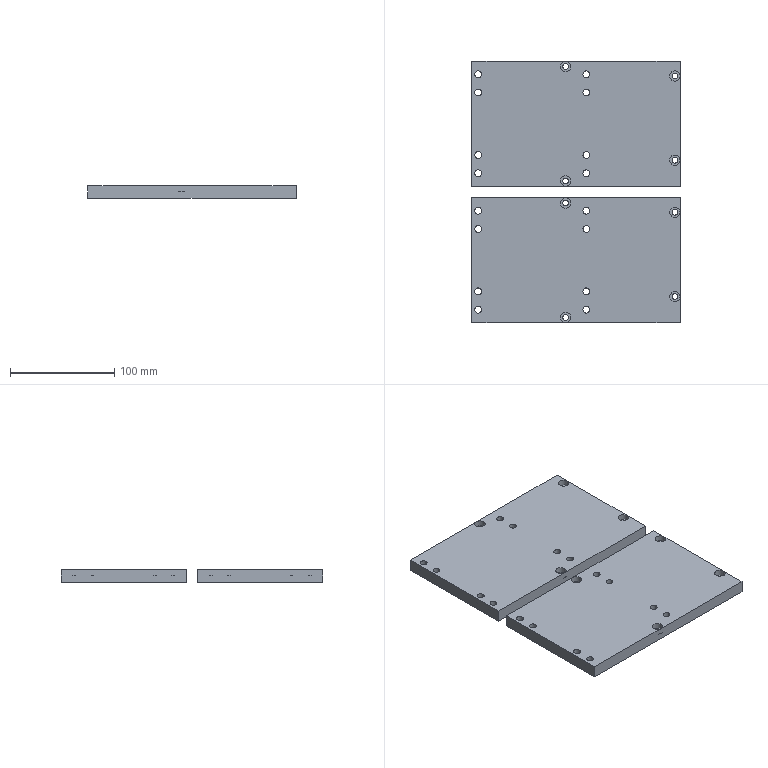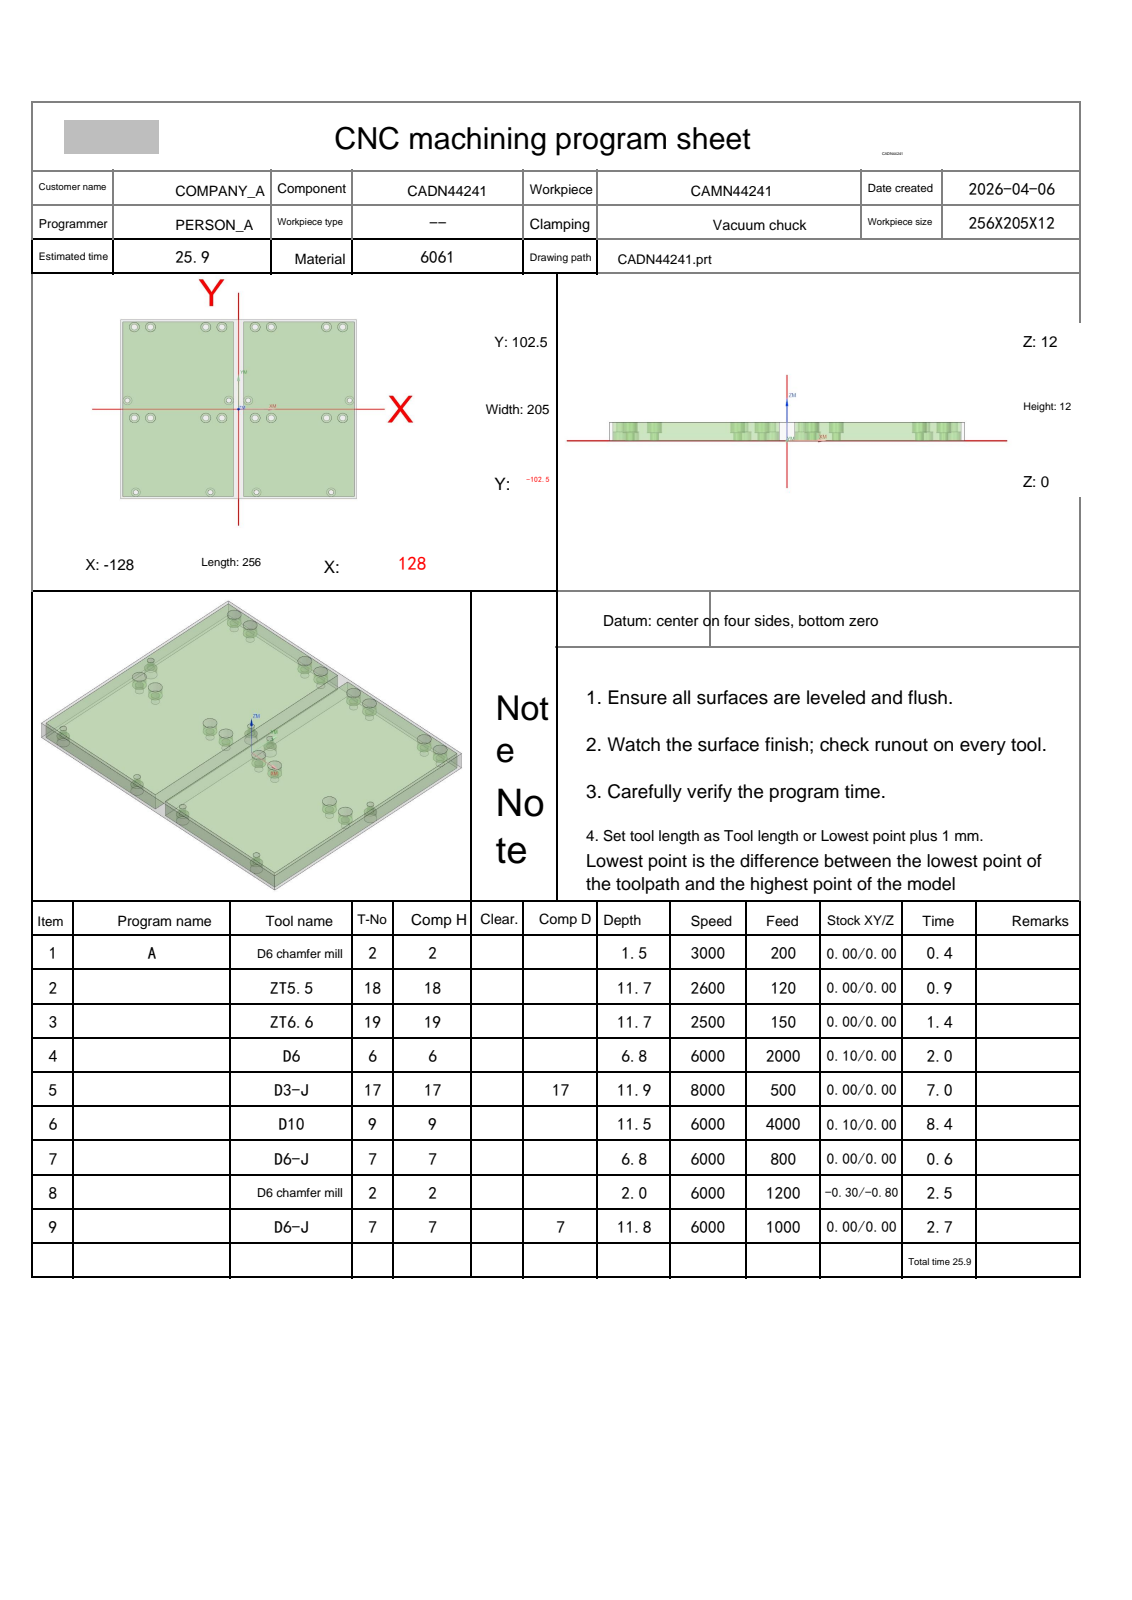NC program | NX | posted by the shop | part box 200 x 251 x 12 mm
Lines 558 to 1452 of 3499:
N5 T17 M06
(D3-J  D=3. R=0. H=17 ce=0.00 di=0.00)
G00 G90 G54 X114.147 Y-8.656 M03 S8000
G43 H17 Z32.
M08
Z5.7
G01 X114.118 Y-8.628 Z5.698 F500.
X113.819 Y-8.431 Z5.679
X113.486 Y-8.298 Z5.66
X113.133 Y-8.235 Z5.642
X112.867 Z5.628
X112.514 Y-8.298 Z5.609
X112.181 Y-8.431 Z5.59
X111.882 Y-8.628 Z5.571
X111.628 Y-8.882 Z5.552
X111.431 Y-9.181 Z5.534
X111.298 Y-9.514 Z5.515
X111.235 Y-9.867 Z5.496
Y-10.133 Z5.482
X111.298 Y-10.486 Z5.463
X111.431 Y-10.819 Z5.445
X111.628 Y-11.118 Z5.426
X111.882 Y-11.372 Z5.407
X112.181 Y-11.569 Z5.388
X112.514 Y-11.702 Z5.369
X112.867 Y-11.765 Z5.351
X113.133 Z5.337
X113.481 Y-11.703 Z5.318
X113.81 Y-11.574 Z5.3
X114.107 Y-11.381 Z5.281
X114.359 Y-11.134 Z5.263
X114.557 Y-10.841 Z5.244
X114.693 Y-10.515 Z5.225
X114.762 Y-10.168 Z5.207
X114.765 Y-10.035 Z5.2
G41 D17
X114.8 Y-10.
G03 X113. Y-8.2 Z5.126 I-1.8 J0.0
X111.2 Y-10. Z5.051 I0.0 J-1.8
X113. Y-11.8 Z4.977 I1.8 J0.0
X114.8 Y-10. Z4.903 I0.0 J1.8
X113. Y-8.2 Z4.829 I-1.8 J0.0
X111.2 Y-10. Z4.754 I0.0 J-1.8
X113. Y-11.8 Z4.68 I1.8 J0.0
X114.8 Y-10. Z4.606 I0.0 J1.8
X113. Y-8.2 Z4.532 I-1.8 J0.0
X111.2 Y-10. Z4.457 I0.0 J-1.8
X113. Y-11.8 Z4.383 I1.8 J0.0
X114.8 Y-10. Z4.309 I0.0 J1.8
X113. Y-8.2 Z4.235 I-1.8 J0.0
X111.2 Y-10. Z4.16 I0.0 J-1.8
X113. Y-11.8 Z4.086 I1.8 J0.0
X114.8 Y-10. Z4.012 I0.0 J1.8
X113. Y-8.2 Z3.938 I-1.8 J0.0
X111.2 Y-10. Z3.863 I0.0 J-1.8
X113. Y-11.8 Z3.789 I1.8 J0.0
X114.8 Y-10. Z3.715 I0.0 J1.8
X113. Y-8.2 Z3.64 I-1.8 J0.0
X111.2 Y-10. Z3.566 I0.0 J-1.8
X113. Y-11.8 Z3.492 I1.8 J0.0
X114.8 Y-10. Z3.418 I0.0 J1.8
X113. Y-8.2 Z3.343 I-1.8 J0.0
X111.2 Y-10. Z3.269 I0.0 J-1.8
X113. Y-11.8 Z3.195 I1.8 J0.0
X114.8 Y-10. Z3.121 I0.0 J1.8
X113. Y-8.2 Z3.046 I-1.8 J0.0
X111.2 Y-10. Z2.972 I0.0 J-1.8
X113. Y-11.8 Z2.898 I1.8 J0.0
X114.8 Y-10. Z2.824 I0.0 J1.8
X113. Y-8.2 Z2.749 I-1.8 J0.0
X111.2 Y-10. Z2.675 I0.0 J-1.8
X113. Y-11.8 Z2.601 I1.8 J0.0
X114.8 Y-10. Z2.526 I0.0 J1.8
X113. Y-8.2 Z2.452 I-1.8 J0.0
X111.2 Y-10. Z2.378 I0.0 J-1.8
X113. Y-11.8 Z2.304 I1.8 J0.0
X114.8 Y-10. Z2.229 I0.0 J1.8
X113. Y-8.2 Z2.155 I-1.8 J0.0
X111.2 Y-10. Z2.081 I0.0 J-1.8
X113. Y-11.8 Z2.007 I1.8 J0.0
X114.8 Y-10. Z1.932 I0.0 J1.8
X113. Y-8.2 Z1.858 I-1.8 J0.0
X111.2 Y-10. Z1.784 I0.0 J-1.8
X113. Y-11.8 Z1.71 I1.8 J0.0
X114.8 Y-10. Z1.635 I0.0 J1.8
X113. Y-8.2 Z1.561 I-1.8 J0.0
X111.2 Y-10. Z1.487 I0.0 J-1.8
X113. Y-11.8 Z1.413 I1.8 J0.0
X114.8 Y-10. Z1.338 I0.0 J1.8
X113. Y-8.2 Z1.264 I-1.8 J0.0
X111.2 Y-10. Z1.19 I0.0 J-1.8
X113. Y-11.8 Z1.115 I1.8 J0.0
X114.8 Y-10. Z1.041 I0.0 J1.8
X113. Y-8.2 Z.967 I-1.8 J0.0
X111.2 Y-10. Z.893 I0.0 J-1.8
X113. Y-11.8 Z.818 I1.8 J0.0
X114.8 Y-10. Z.744 I0.0 J1.8
X113. Y-8.2 Z.67 I-1.8 J0.0
X111.2 Y-10. Z.596 I0.0 J-1.8
X113. Y-11.8 Z.521 I1.8 J0.0
X114.8 Y-10. Z.447 I0.0 J1.8
X113. Y-8.2 Z.373 I-1.8 J0.0
X111.2 Y-10. Z.299 I0.0 J-1.8
X113. Y-11.8 Z.224 I1.8 J0.0
X114.8 Y-10. Z.15 I0.0 J1.8
X113. Y-8.2 I-1.8 J0.0
X111.2 Y-10. I0.0 J-1.8
X113. Y-11.8 I1.8 J0.0
X114.8 Y-10. I0.0 J1.8
X114.756 Y-9.603 I-1.8 J0.0
G01 X114.747 Y-9.577
X114.723 Y-9.562
X114.696 Y-9.566
G40 X114.647 Y-9.577
Z1.15
G00 Z32.
X96.647 Y-8.656
Z5.7
G01 X96.618 Y-8.628 Z5.698
X96.319 Y-8.431 Z5.679
X95.986 Y-8.298 Z5.66
X95.633 Y-8.235 Z5.642
X95.367 Z5.628
X95.014 Y-8.298 Z5.609
X94.681 Y-8.431 Z5.59
X94.382 Y-8.628 Z5.571
X94.128 Y-8.882 Z5.552
X93.931 Y-9.181 Z5.534
X93.798 Y-9.514 Z5.515
X93.735 Y-9.867 Z5.496
Y-10.133 Z5.482
X93.798 Y-10.486 Z5.463
X93.931 Y-10.819 Z5.445
X94.128 Y-11.118 Z5.426
X94.382 Y-11.372 Z5.407
X94.681 Y-11.569 Z5.388
X95.014 Y-11.702 Z5.369
X95.367 Y-11.765 Z5.351
X95.633 Z5.337
X95.981 Y-11.703 Z5.318
X96.31 Y-11.574 Z5.3
X96.607 Y-11.381 Z5.281
X96.859 Y-11.134 Z5.263
X97.057 Y-10.841 Z5.244
X97.193 Y-10.515 Z5.225
X97.262 Y-10.168 Z5.207
X97.265 Y-10.035 Z5.2
G41 D17
X97.3 Y-10.
G03 X95.5 Y-8.2 Z5.126 I-1.8 J0.0
X93.7 Y-10. Z5.051 I0.0 J-1.8
X95.5 Y-11.8 Z4.977 I1.8 J0.0
X97.3 Y-10. Z4.903 I0.0 J1.8
X95.5 Y-8.2 Z4.829 I-1.8 J0.0
X93.7 Y-10. Z4.754 I0.0 J-1.8
X95.5 Y-11.8 Z4.68 I1.8 J0.0
X97.3 Y-10. Z4.606 I0.0 J1.8
X95.5 Y-8.2 Z4.532 I-1.8 J0.0
X93.7 Y-10. Z4.457 I0.0 J-1.8
X95.5 Y-11.8 Z4.383 I1.8 J0.0
X97.3 Y-10. Z4.309 I0.0 J1.8
X95.5 Y-8.2 Z4.235 I-1.8 J0.0
X93.7 Y-10. Z4.16 I0.0 J-1.8
X95.5 Y-11.8 Z4.086 I1.8 J0.0
X97.3 Y-10. Z4.012 I0.0 J1.8
X95.5 Y-8.2 Z3.938 I-1.8 J0.0
X93.7 Y-10. Z3.863 I0.0 J-1.8
X95.5 Y-11.8 Z3.789 I1.8 J0.0
X97.3 Y-10. Z3.715 I0.0 J1.8
X95.5 Y-8.2 Z3.64 I-1.8 J0.0
X93.7 Y-10. Z3.566 I0.0 J-1.8
X95.5 Y-11.8 Z3.492 I1.8 J0.0
X97.3 Y-10. Z3.418 I0.0 J1.8
X95.5 Y-8.2 Z3.343 I-1.8 J0.0
X93.7 Y-10. Z3.269 I0.0 J-1.8
X95.5 Y-11.8 Z3.195 I1.8 J0.0
X97.3 Y-10. Z3.121 I0.0 J1.8
X95.5 Y-8.2 Z3.046 I-1.8 J0.0
X93.7 Y-10. Z2.972 I0.0 J-1.8
X95.5 Y-11.8 Z2.898 I1.8 J0.0
X97.3 Y-10. Z2.824 I0.0 J1.8
X95.5 Y-8.2 Z2.749 I-1.8 J0.0
X93.7 Y-10. Z2.675 I0.0 J-1.8
X95.5 Y-11.8 Z2.601 I1.8 J0.0
X97.3 Y-10. Z2.526 I0.0 J1.8
X95.5 Y-8.2 Z2.452 I-1.8 J0.0
X93.7 Y-10. Z2.378 I0.0 J-1.8
X95.5 Y-11.8 Z2.304 I1.8 J0.0
X97.3 Y-10. Z2.229 I0.0 J1.8
X95.5 Y-8.2 Z2.155 I-1.8 J0.0
X93.7 Y-10. Z2.081 I0.0 J-1.8
X95.5 Y-11.8 Z2.007 I1.8 J0.0
X97.3 Y-10. Z1.932 I0.0 J1.8
X95.5 Y-8.2 Z1.858 I-1.8 J0.0
X93.7 Y-10. Z1.784 I0.0 J-1.8
X95.5 Y-11.8 Z1.71 I1.8 J0.0
X97.3 Y-10. Z1.635 I0.0 J1.8
X95.5 Y-8.2 Z1.561 I-1.8 J0.0
X93.7 Y-10. Z1.487 I0.0 J-1.8
X95.5 Y-11.8 Z1.413 I1.8 J0.0
X97.3 Y-10. Z1.338 I0.0 J1.8
X95.5 Y-8.2 Z1.264 I-1.8 J0.0
X93.7 Y-10. Z1.19 I0.0 J-1.8
X95.5 Y-11.8 Z1.115 I1.8 J0.0
X97.3 Y-10. Z1.041 I0.0 J1.8
X95.5 Y-8.2 Z.967 I-1.8 J0.0
X93.7 Y-10. Z.893 I0.0 J-1.8
X95.5 Y-11.8 Z.818 I1.8 J0.0
X97.3 Y-10. Z.744 I0.0 J1.8
X95.5 Y-8.2 Z.67 I-1.8 J0.0
X93.7 Y-10. Z.596 I0.0 J-1.8
X95.5 Y-11.8 Z.521 I1.8 J0.0
X97.3 Y-10. Z.447 I0.0 J1.8
X95.5 Y-8.2 Z.373 I-1.8 J0.0
X93.7 Y-10. Z.299 I0.0 J-1.8
X95.5 Y-11.8 Z.224 I1.8 J0.0
X97.3 Y-10. Z.15 I0.0 J1.8
X95.5 Y-8.2 I-1.8 J0.0
X93.7 Y-10. I0.0 J-1.8
X95.5 Y-11.8 I1.8 J0.0
X97.3 Y-10. I0.0 J1.8
X97.256 Y-9.603 I-1.8 J0.0
G01 X97.247 Y-9.577
X97.223 Y-9.562
X97.196 Y-9.566
G40 X97.147 Y-9.577
Z1.15
G00 Z32.
X36.647 Y-8.656
Z5.7
G01 X36.618 Y-8.628 Z5.698
X36.319 Y-8.431 Z5.679
X35.986 Y-8.298 Z5.66
X35.633 Y-8.235 Z5.642
X35.367 Z5.628
X35.014 Y-8.298 Z5.609
X34.681 Y-8.431 Z5.59
X34.382 Y-8.628 Z5.571
X34.128 Y-8.882 Z5.552
X33.931 Y-9.181 Z5.534
X33.798 Y-9.514 Z5.515
X33.735 Y-9.867 Z5.496
Y-10.133 Z5.482
X33.798 Y-10.486 Z5.463
X33.931 Y-10.819 Z5.445
X34.128 Y-11.118 Z5.426
X34.382 Y-11.372 Z5.407
X34.681 Y-11.569 Z5.388
X35.014 Y-11.702 Z5.369
X35.367 Y-11.765 Z5.351
X35.633 Z5.337
X35.981 Y-11.703 Z5.318
X36.31 Y-11.574 Z5.3
X36.607 Y-11.381 Z5.281
X36.859 Y-11.134 Z5.263
X37.057 Y-10.841 Z5.244
X37.193 Y-10.515 Z5.225
X37.262 Y-10.168 Z5.207
X37.265 Y-10.035 Z5.2
G41 D17
X37.3 Y-10.
G03 X35.5 Y-8.2 Z5.126 I-1.8 J0.0
X33.7 Y-10. Z5.051 I0.0 J-1.8
X35.5 Y-11.8 Z4.977 I1.8 J0.0
X37.3 Y-10. Z4.903 I0.0 J1.8
X35.5 Y-8.2 Z4.829 I-1.8 J0.0
X33.7 Y-10. Z4.754 I0.0 J-1.8
X35.5 Y-11.8 Z4.68 I1.8 J0.0
X37.3 Y-10. Z4.606 I0.0 J1.8
X35.5 Y-8.2 Z4.532 I-1.8 J0.0
X33.7 Y-10. Z4.457 I0.0 J-1.8
X35.5 Y-11.8 Z4.383 I1.8 J0.0
X37.3 Y-10. Z4.309 I0.0 J1.8
X35.5 Y-8.2 Z4.235 I-1.8 J0.0
X33.7 Y-10. Z4.16 I0.0 J-1.8
X35.5 Y-11.8 Z4.086 I1.8 J0.0
X37.3 Y-10. Z4.012 I0.0 J1.8
X35.5 Y-8.2 Z3.938 I-1.8 J0.0
X33.7 Y-10. Z3.863 I0.0 J-1.8
X35.5 Y-11.8 Z3.789 I1.8 J0.0
X37.3 Y-10. Z3.715 I0.0 J1.8
X35.5 Y-8.2 Z3.64 I-1.8 J0.0
X33.7 Y-10. Z3.566 I0.0 J-1.8
X35.5 Y-11.8 Z3.492 I1.8 J0.0
X37.3 Y-10. Z3.418 I0.0 J1.8
X35.5 Y-8.2 Z3.343 I-1.8 J0.0
X33.7 Y-10. Z3.269 I0.0 J-1.8
X35.5 Y-11.8 Z3.195 I1.8 J0.0
X37.3 Y-10. Z3.121 I0.0 J1.8
X35.5 Y-8.2 Z3.046 I-1.8 J0.0
X33.7 Y-10. Z2.972 I0.0 J-1.8
X35.5 Y-11.8 Z2.898 I1.8 J0.0
X37.3 Y-10. Z2.824 I0.0 J1.8
X35.5 Y-8.2 Z2.749 I-1.8 J0.0
X33.7 Y-10. Z2.675 I0.0 J-1.8
X35.5 Y-11.8 Z2.601 I1.8 J0.0
X37.3 Y-10. Z2.526 I0.0 J1.8
X35.5 Y-8.2 Z2.452 I-1.8 J0.0
X33.7 Y-10. Z2.378 I0.0 J-1.8
X35.5 Y-11.8 Z2.304 I1.8 J0.0
X37.3 Y-10. Z2.229 I0.0 J1.8
X35.5 Y-8.2 Z2.155 I-1.8 J0.0
X33.7 Y-10. Z2.081 I0.0 J-1.8
X35.5 Y-11.8 Z2.007 I1.8 J0.0
X37.3 Y-10. Z1.932 I0.0 J1.8
X35.5 Y-8.2 Z1.858 I-1.8 J0.0
X33.7 Y-10. Z1.784 I0.0 J-1.8
X35.5 Y-11.8 Z1.71 I1.8 J0.0
X37.3 Y-10. Z1.635 I0.0 J1.8
X35.5 Y-8.2 Z1.561 I-1.8 J0.0
X33.7 Y-10. Z1.487 I0.0 J-1.8
X35.5 Y-11.8 Z1.413 I1.8 J0.0
X37.3 Y-10. Z1.338 I0.0 J1.8
X35.5 Y-8.2 Z1.264 I-1.8 J0.0
X33.7 Y-10. Z1.19 I0.0 J-1.8
X35.5 Y-11.8 Z1.115 I1.8 J0.0
X37.3 Y-10. Z1.041 I0.0 J1.8
X35.5 Y-8.2 Z.967 I-1.8 J0.0
X33.7 Y-10. Z.893 I0.0 J-1.8
X35.5 Y-11.8 Z.818 I1.8 J0.0
X37.3 Y-10. Z.744 I0.0 J1.8
X35.5 Y-8.2 Z.67 I-1.8 J0.0
X33.7 Y-10. Z.596 I0.0 J-1.8
X35.5 Y-11.8 Z.521 I1.8 J0.0
X37.3 Y-10. Z.447 I0.0 J1.8
X35.5 Y-8.2 Z.373 I-1.8 J0.0
X33.7 Y-10. Z.299 I0.0 J-1.8
X35.5 Y-11.8 Z.224 I1.8 J0.0
X37.3 Y-10. Z.15 I0.0 J1.8
X35.5 Y-8.2 I-1.8 J0.0
X33.7 Y-10. I0.0 J-1.8
X35.5 Y-11.8 I1.8 J0.0
X37.3 Y-10. I0.0 J1.8
X37.256 Y-9.603 I-1.8 J0.0
G01 X37.247 Y-9.577
X37.223 Y-9.562
X37.196 Y-9.566
G40 X37.147 Y-9.577
Z1.15
G00 Z32.
X19.344 Y-11.147
Z5.7
G01 X19.372 Y-11.118 Z5.698
X19.569 Y-10.819 Z5.679
X19.702 Y-10.486 Z5.66
X19.765 Y-10.133 Z5.642
Y-9.867 Z5.628
X19.702 Y-9.514 Z5.609
X19.569 Y-9.181 Z5.59
X19.372 Y-8.882 Z5.571
X19.118 Y-8.628 Z5.552
X18.819 Y-8.431 Z5.534
X18.486 Y-8.298 Z5.515
X18.133 Y-8.235 Z5.496
X17.867 Z5.482
X17.514 Y-8.298 Z5.463
X17.181 Y-8.431 Z5.445
X16.882 Y-8.628 Z5.426
X16.628 Y-8.882 Z5.407
X16.431 Y-9.181 Z5.388
X16.298 Y-9.514 Z5.369
X16.235 Y-9.867 Z5.351
Y-10.133 Z5.337
X16.297 Y-10.481 Z5.318
X16.426 Y-10.81 Z5.3
X16.619 Y-11.107 Z5.281
X16.866 Y-11.359 Z5.263
X17.159 Y-11.557 Z5.244
X17.485 Y-11.693 Z5.225
X17.832 Y-11.762 Z5.207
X17.965 Y-11.765 Z5.2
G41 D17
X18. Y-11.8
G03 X19.8 Y-10. Z5.126 I0.0 J1.8
X18. Y-8.2 Z5.051 I-1.8 J0.0
X16.2 Y-10. Z4.977 I0.0 J-1.8
X18. Y-11.8 Z4.903 I1.8 J0.0
X19.8 Y-10. Z4.829 I0.0 J1.8
X18. Y-8.2 Z4.754 I-1.8 J0.0
X16.2 Y-10. Z4.68 I0.0 J-1.8
X18. Y-11.8 Z4.606 I1.8 J0.0
X19.8 Y-10. Z4.532 I0.0 J1.8
X18. Y-8.2 Z4.457 I-1.8 J0.0
X16.2 Y-10. Z4.383 I0.0 J-1.8
X18. Y-11.8 Z4.309 I1.8 J0.0
X19.8 Y-10. Z4.235 I0.0 J1.8
X18. Y-8.2 Z4.16 I-1.8 J0.0
X16.2 Y-10. Z4.086 I0.0 J-1.8
X18. Y-11.8 Z4.012 I1.8 J0.0
X19.8 Y-10. Z3.938 I0.0 J1.8
X18. Y-8.2 Z3.863 I-1.8 J0.0
X16.2 Y-10. Z3.789 I0.0 J-1.8
X18. Y-11.8 Z3.715 I1.8 J0.0
X19.8 Y-10. Z3.64 I0.0 J1.8
X18. Y-8.2 Z3.566 I-1.8 J0.0
X16.2 Y-10. Z3.492 I0.0 J-1.8
X18. Y-11.8 Z3.418 I1.8 J0.0
X19.8 Y-10. Z3.343 I0.0 J1.8
X18. Y-8.2 Z3.269 I-1.8 J0.0
X16.2 Y-10. Z3.195 I0.0 J-1.8
X18. Y-11.8 Z3.121 I1.8 J0.0
X19.8 Y-10. Z3.046 I0.0 J1.8
X18. Y-8.2 Z2.972 I-1.8 J0.0
X16.2 Y-10. Z2.898 I0.0 J-1.8
X18. Y-11.8 Z2.824 I1.8 J0.0
X19.8 Y-10. Z2.749 I0.0 J1.8
X18. Y-8.2 Z2.675 I-1.8 J0.0
X16.2 Y-10. Z2.601 I0.0 J-1.8
X18. Y-11.8 Z2.526 I1.8 J0.0
X19.8 Y-10. Z2.452 I0.0 J1.8
X18. Y-8.2 Z2.378 I-1.8 J0.0
X16.2 Y-10. Z2.304 I0.0 J-1.8
X18. Y-11.8 Z2.229 I1.8 J0.0
X19.8 Y-10. Z2.155 I0.0 J1.8
X18. Y-8.2 Z2.081 I-1.8 J0.0
X16.2 Y-10. Z2.007 I0.0 J-1.8
X18. Y-11.8 Z1.932 I1.8 J0.0
X19.8 Y-10. Z1.858 I0.0 J1.8
X18. Y-8.2 Z1.784 I-1.8 J0.0
X16.2 Y-10. Z1.71 I0.0 J-1.8
X18. Y-11.8 Z1.635 I1.8 J0.0
X19.8 Y-10. Z1.561 I0.0 J1.8
X18. Y-8.2 Z1.487 I-1.8 J0.0
X16.2 Y-10. Z1.413 I0.0 J-1.8
X18. Y-11.8 Z1.338 I1.8 J0.0
X19.8 Y-10. Z1.264 I0.0 J1.8
X18. Y-8.2 Z1.19 I-1.8 J0.0
X16.2 Y-10. Z1.115 I0.0 J-1.8
X18. Y-11.8 Z1.041 I1.8 J0.0
X19.8 Y-10. Z.967 I0.0 J1.8
X18. Y-8.2 Z.893 I-1.8 J0.0
X16.2 Y-10. Z.818 I0.0 J-1.8
X18. Y-11.8 Z.744 I1.8 J0.0
X19.8 Y-10. Z.67 I0.0 J1.8
X18. Y-8.2 Z.596 I-1.8 J0.0
X16.2 Y-10. Z.521 I0.0 J-1.8
X18. Y-11.8 Z.447 I1.8 J0.0
X19.8 Y-10. Z.373 I0.0 J1.8
X18. Y-8.2 Z.299 I-1.8 J0.0
X16.2 Y-10. Z.224 I0.0 J-1.8
X18. Y-11.8 Z.15 I1.8 J0.0
X19.8 Y-10. I0.0 J1.8
X18. Y-8.2 I-1.8 J0.0
X16.2 Y-10. I0.0 J-1.8
X18. Y-11.8 I1.8 J0.0
X18.397 Y-11.756 I0.0 J1.8
G01 X18.423 Y-11.747
X18.438 Y-11.723
X18.434 Y-11.696
G40 X18.423 Y-11.647
Z1.15
G00 Z32.
X-16.656 Y-11.146
Z5.7
G01 X-16.628 Y-11.118 Z5.698
X-16.431 Y-10.819 Z5.679
X-16.298 Y-10.486 Z5.66
X-16.235 Y-10.133 Z5.642
Y-9.867 Z5.628
X-16.298 Y-9.514 Z5.609
X-16.431 Y-9.181 Z5.59
X-16.628 Y-8.882 Z5.571
X-16.882 Y-8.628 Z5.552
X-17.181 Y-8.431 Z5.534
X-17.514 Y-8.298 Z5.515
X-17.867 Y-8.235 Z5.496
X-18.133 Z5.482
X-18.389 Y-8.273 Z5.469
X-18.637 Y-8.349 Z5.455
X-18.872 Y-8.46 Z5.441
X-19.093 Y-8.607 Z5.427
X-19.356 Y-8.863 Z5.408
X-19.561 Y-9.166 Z5.389
X-19.7 Y-9.506 Z5.37
X-19.765 Y-9.867 Z5.351
Y-10.133 Z5.337
X-19.703 Y-10.481 Z5.318
X-19.574 Y-10.81 Z5.3
X-19.381 Y-11.107 Z5.281
X-19.134 Y-11.359 Z5.263
X-18.841 Y-11.557 Z5.244
X-18.515 Y-11.693 Z5.225
X-18.168 Y-11.762 Z5.207
X-18.035 Y-11.765 Z5.2
G41 D17
X-18. Y-11.8
G03 X-16.2 Y-10. Z5.126 I0.0 J1.8
X-18. Y-8.2 Z5.051 I-1.8 J0.0
X-19.002 Y-8.504 Z5.024 I0.0 J-1.8
X-19.8 Y-10. Z4.977 I1.002 J-1.496
X-18. Y-11.8 Z4.903 I1.8 J0.0
X-16.2 Y-10. Z4.829 I0.0 J1.8
X-18. Y-8.2 Z4.754 I-1.8 J0.0
X-19.002 Y-8.504 Z4.727 I0.0 J-1.8
X-19.8 Y-10. Z4.68 I1.002 J-1.496
X-18. Y-11.8 Z4.606 I1.8 J0.0
X-16.2 Y-10. Z4.532 I0.0 J1.8
X-18. Y-8.2 Z4.457 I-1.8 J0.0
X-19.002 Y-8.504 Z4.429 I0.0 J-1.8
X-19.8 Y-10. Z4.383 I1.002 J-1.496
X-18. Y-11.8 Z4.309 I1.8 J0.0
X-16.2 Y-10. Z4.235 I0.0 J1.8
X-18. Y-8.2 Z4.16 I-1.8 J0.0
X-19.002 Y-8.504 Z4.132 I0.0 J-1.8
X-19.8 Y-10. Z4.086 I1.002 J-1.496
X-18. Y-11.8 Z4.012 I1.8 J0.0
X-16.2 Y-10. Z3.938 I0.0 J1.8
X-18. Y-8.2 Z3.863 I-1.8 J0.0
X-19.002 Y-8.504 Z3.835 I0.0 J-1.8
X-19.8 Y-10. Z3.789 I1.002 J-1.496
X-18. Y-11.8 Z3.715 I1.8 J0.0
X-16.2 Y-10. Z3.64 I0.0 J1.8
X-18. Y-8.2 Z3.566 I-1.8 J0.0
X-19.002 Y-8.504 Z3.538 I0.0 J-1.8
X-19.8 Y-10. Z3.492 I1.002 J-1.496
X-18. Y-11.8 Z3.418 I1.8 J0.0
X-16.2 Y-10. Z3.343 I0.0 J1.8
X-18. Y-8.2 Z3.269 I-1.8 J0.0
X-19.002 Y-8.504 Z3.241 I0.0 J-1.8
X-19.8 Y-10. Z3.195 I1.002 J-1.496
X-18. Y-11.8 Z3.121 I1.8 J0.0
X-16.2 Y-10. Z3.046 I0.0 J1.8
X-18. Y-8.2 Z2.972 I-1.8 J0.0
X-19.002 Y-8.504 Z2.944 I0.0 J-1.8
X-19.8 Y-10. Z2.898 I1.002 J-1.496
X-18. Y-11.8 Z2.824 I1.8 J0.0
X-16.2 Y-10. Z2.749 I0.0 J1.8
X-18. Y-8.2 Z2.675 I-1.8 J0.0
X-19.002 Y-8.504 Z2.647 I0.0 J-1.8
X-19.8 Y-10. Z2.601 I1.002 J-1.496
X-18. Y-11.8 Z2.526 I1.8 J0.0
X-16.2 Y-10. Z2.452 I0.0 J1.8
X-18. Y-8.2 Z2.378 I-1.8 J0.0
X-19.002 Y-8.504 Z2.35 I0.0 J-1.8
X-19.8 Y-10. Z2.304 I1.002 J-1.496
X-18. Y-11.8 Z2.229 I1.8 J0.0
X-16.2 Y-10. Z2.155 I0.0 J1.8
X-18. Y-8.2 Z2.081 I-1.8 J0.0
X-19.002 Y-8.504 Z2.053 I0.0 J-1.8
X-19.8 Y-10. Z2.007 I1.002 J-1.496
X-18. Y-11.8 Z1.932 I1.8 J0.0
X-16.2 Y-10. Z1.858 I0.0 J1.8
X-18. Y-8.2 Z1.784 I-1.8 J0.0
X-19.002 Y-8.504 Z1.756 I0.0 J-1.8
X-19.8 Y-10. Z1.71 I1.002 J-1.496
X-18. Y-11.8 Z1.635 I1.8 J0.0
X-16.2 Y-10. Z1.561 I0.0 J1.8
X-18. Y-8.2 Z1.487 I-1.8 J0.0
X-19.002 Y-8.504 Z1.459 I0.0 J-1.8
X-19.8 Y-10. Z1.413 I1.002 J-1.496
X-18. Y-11.8 Z1.338 I1.8 J0.0
X-16.2 Y-10. Z1.264 I0.0 J1.8
X-18. Y-8.2 Z1.19 I-1.8 J0.0
X-19.002 Y-8.504 Z1.162 I0.0 J-1.8
X-19.8 Y-10. Z1.115 I1.002 J-1.496
X-18. Y-11.8 Z1.041 I1.8 J0.0
X-16.2 Y-10. Z.967 I0.0 J1.8
X-18. Y-8.2 Z.893 I-1.8 J0.0
X-19.002 Y-8.504 Z.865 I0.0 J-1.8
X-19.8 Y-10. Z.818 I1.002 J-1.496
X-18. Y-11.8 Z.744 I1.8 J0.0
X-16.2 Y-10. Z.67 I0.0 J1.8
X-18. Y-8.2 Z.596 I-1.8 J0.0
X-19.002 Y-8.504 Z.568 I0.0 J-1.8
X-19.8 Y-10. Z.521 I1.002 J-1.496
X-18. Y-11.8 Z.447 I1.8 J0.0
X-16.2 Y-10. Z.373 I0.0 J1.8
X-18. Y-8.2 Z.299 I-1.8 J0.0
X-19.002 Y-8.504 Z.271 I0.0 J-1.8
X-19.8 Y-10. Z.224 I1.002 J-1.496
X-18. Y-11.8 Z.15 I1.8 J0.0
X-16.2 Y-10. I0.0 J1.8
X-18. Y-8.2 I-1.8 J0.0
X-19.8 Y-10. I0.0 J-1.8
X-18. Y-11.8 I1.8 J0.0
X-17.603 Y-11.756 I0.0 J1.8
G01 X-17.577 Y-11.747
X-17.562 Y-11.723
X-17.566 Y-11.696
G40 X-17.577 Y-11.647
Z1.15
G00 Z32.
X-34.156 Y-11.147
Z5.7
G01 X-34.128 Y-11.118 Z5.698
X-33.931 Y-10.819 Z5.679
X-33.798 Y-10.486 Z5.66
X-33.735 Y-10.133 Z5.642
Y-9.867 Z5.628
X-33.798 Y-9.514 Z5.609
X-33.931 Y-9.181 Z5.59
X-34.128 Y-8.882 Z5.571
X-34.382 Y-8.628 Z5.552
X-34.681 Y-8.431 Z5.534
X-35.014 Y-8.298 Z5.515
X-35.367 Y-8.235 Z5.496
X-35.633 Z5.482
X-35.986 Y-8.298 Z5.463
X-36.319 Y-8.431 Z5.445
X-36.618 Y-8.628 Z5.426
X-36.872 Y-8.882 Z5.407
X-37.069 Y-9.181 Z5.388
X-37.202 Y-9.514 Z5.369
X-37.265 Y-9.867 Z5.351
Y-10.133 Z5.337
X-37.203 Y-10.481 Z5.318
X-37.074 Y-10.81 Z5.3
X-36.881 Y-11.107 Z5.281
X-36.634 Y-11.359 Z5.263
X-36.341 Y-11.557 Z5.244
X-36.015 Y-11.693 Z5.225
X-35.668 Y-11.762 Z5.207
X-35.535 Y-11.765 Z5.2
G41 D17
X-35.5 Y-11.8
G03 X-33.7 Y-10. Z5.126 I0.0 J1.8
X-35.5 Y-8.2 Z5.051 I-1.8 J0.0
X-37.3 Y-10. Z4.977 I0.0 J-1.8
X-35.5 Y-11.8 Z4.903 I1.8 J0.0
X-33.7 Y-10. Z4.829 I0.0 J1.8
X-35.5 Y-8.2 Z4.754 I-1.8 J0.0
X-37.3 Y-10. Z4.68 I0.0 J-1.8
X-35.5 Y-11.8 Z4.606 I1.8 J0.0
X-33.7 Y-10. Z4.532 I0.0 J1.8
X-35.5 Y-8.2 Z4.457 I-1.8 J0.0
X-37.3 Y-10. Z4.383 I0.0 J-1.8
X-35.5 Y-11.8 Z4.309 I1.8 J0.0
X-33.7 Y-10. Z4.235 I0.0 J1.8
X-35.5 Y-8.2 Z4.16 I-1.8 J0.0
X-37.3 Y-10. Z4.086 I0.0 J-1.8
X-35.5 Y-11.8 Z4.012 I1.8 J0.0
X-33.7 Y-10. Z3.938 I0.0 J1.8
X-35.5 Y-8.2 Z3.863 I-1.8 J0.0
X-37.3 Y-10. Z3.789 I0.0 J-1.8
X-35.5 Y-11.8 Z3.715 I1.8 J0.0
X-33.7 Y-10. Z3.64 I0.0 J1.8
X-35.5 Y-8.2 Z3.566 I-1.8 J0.0
X-37.3 Y-10. Z3.492 I0.0 J-1.8
X-35.5 Y-11.8 Z3.418 I1.8 J0.0
X-33.7 Y-10. Z3.343 I0.0 J1.8
X-35.5 Y-8.2 Z3.269 I-1.8 J0.0
X-37.3 Y-10. Z3.195 I0.0 J-1.8
X-35.5 Y-11.8 Z3.121 I1.8 J0.0
X-33.7 Y-10. Z3.046 I0.0 J1.8
X-35.5 Y-8.2 Z2.972 I-1.8 J0.0
X-37.3 Y-10. Z2.898 I0.0 J-1.8
X-35.5 Y-11.8 Z2.824 I1.8 J0.0
X-33.7 Y-10. Z2.749 I0.0 J1.8
X-35.5 Y-8.2 Z2.675 I-1.8 J0.0
X-37.3 Y-10. Z2.601 I0.0 J-1.8
X-35.5 Y-11.8 Z2.526 I1.8 J0.0
X-33.7 Y-10. Z2.452 I0.0 J1.8
X-35.5 Y-8.2 Z2.378 I-1.8 J0.0
X-37.3 Y-10. Z2.304 I0.0 J-1.8
X-35.5 Y-11.8 Z2.229 I1.8 J0.0
X-33.7 Y-10. Z2.155 I0.0 J1.8
X-35.5 Y-8.2 Z2.081 I-1.8 J0.0
X-37.3 Y-10. Z2.007 I0.0 J-1.8
X-35.5 Y-11.8 Z1.932 I1.8 J0.0
X-33.7 Y-10. Z1.858 I0.0 J1.8
X-35.5 Y-8.2 Z1.784 I-1.8 J0.0
X-37.3 Y-10. Z1.71 I0.0 J-1.8
X-35.5 Y-11.8 Z1.635 I1.8 J0.0
X-33.7 Y-10. Z1.561 I0.0 J1.8
X-35.5 Y-8.2 Z1.487 I-1.8 J0.0
X-37.3 Y-10. Z1.413 I0.0 J-1.8
X-35.5 Y-11.8 Z1.338 I1.8 J0.0
X-33.7 Y-10. Z1.264 I0.0 J1.8
X-35.5 Y-8.2 Z1.19 I-1.8 J0.0
X-37.3 Y-10. Z1.115 I0.0 J-1.8
X-35.5 Y-11.8 Z1.041 I1.8 J0.0
X-33.7 Y-10. Z.967 I0.0 J1.8
X-35.5 Y-8.2 Z.893 I-1.8 J0.0
X-37.3 Y-10. Z.818 I0.0 J-1.8
X-35.5 Y-11.8 Z.744 I1.8 J0.0
X-33.7 Y-10. Z.67 I0.0 J1.8
X-35.5 Y-8.2 Z.596 I-1.8 J0.0
X-37.3 Y-10. Z.521 I0.0 J-1.8
X-35.5 Y-11.8 Z.447 I1.8 J0.0
X-33.7 Y-10. Z.373 I0.0 J1.8
X-35.5 Y-8.2 Z.299 I-1.8 J0.0
X-37.3 Y-10. Z.224 I0.0 J-1.8
X-35.5 Y-11.8 Z.15 I1.8 J0.0
X-33.7 Y-10. I0.0 J1.8
X-35.5 Y-8.2 I-1.8 J0.0
X-37.3 Y-10. I0.0 J-1.8
X-35.5 Y-11.8 I1.8 J0.0
X-35.103 Y-11.756 I0.0 J1.8
G01 X-35.077 Y-11.747
X-35.062 Y-11.723
X-35.066 Y-11.696
G40 X-35.077 Y-11.647
Z1.15
G00 Z32.
X-96.647 Y-11.344
Z5.7
G01 X-96.618 Y-11.372 Z5.698
X-96.319 Y-11.569 Z5.679
X-95.986 Y-11.702 Z5.66
X-95.633 Y-11.765 Z5.642
X-95.367 Z5.628
X-95.014 Y-11.702 Z5.609
X-94.681 Y-11.569 Z5.59
X-94.382 Y-11.372 Z5.571
X-94.128 Y-11.118 Z5.552
X-93.931 Y-10.819 Z5.534
X-93.798 Y-10.486 Z5.515
X-93.735 Y-10.133 Z5.496
Y-9.867 Z5.482
X-93.798 Y-9.514 Z5.463
X-93.931 Y-9.181 Z5.445
X-94.128 Y-8.882 Z5.426
X-94.382 Y-8.628 Z5.407
X-94.681 Y-8.431 Z5.388
X-95.014 Y-8.298 Z5.369
X-95.367 Y-8.235 Z5.351
X-95.633 Z5.337
X-95.981 Y-8.297 Z5.318
X-96.31 Y-8.426 Z5.3
X-96.607 Y-8.619 Z5.281
X-96.859 Y-8.866 Z5.263
X-97.057 Y-9.159 Z5.244
X-97.193 Y-9.485 Z5.225
X-97.262 Y-9.832 Z5.207
X-97.265 Y-9.965 Z5.2
G41 D17
X-97.3 Y-10.
G03 X-95.5 Y-11.8 Z5.126 I1.8 J0.0
X-93.7 Y-10. Z5.051 I0.0 J1.8
X-95.5 Y-8.2 Z4.977 I-1.8 J0.0
X-97.3 Y-10. Z4.903 I0.0 J-1.8
X-95.5 Y-11.8 Z4.829 I1.8 J0.0
X-93.7 Y-10. Z4.754 I0.0 J1.8
X-95.5 Y-8.2 Z4.68 I-1.8 J0.0
X-97.3 Y-10. Z4.606 I0.0 J-1.8
X-95.5 Y-11.8 Z4.532 I1.8 J0.0
X-93.7 Y-10. Z4.457 I0.0 J1.8
X-95.5 Y-8.2 Z4.383 I-1.8 J0.0
X-97.3 Y-10. Z4.309 I0.0 J-1.8
X-95.5 Y-11.8 Z4.235 I1.8 J0.0
X-93.7 Y-10. Z4.16 I0.0 J1.8
X-95.5 Y-8.2 Z4.086 I-1.8 J0.0
X-97.3 Y-10. Z4.012 I0.0 J-1.8
X-95.5 Y-11.8 Z3.938 I1.8 J0.0
X-93.7 Y-10. Z3.863 I0.0 J1.8
X-95.5 Y-8.2 Z3.789 I-1.8 J0.0
X-97.3 Y-10. Z3.715 I0.0 J-1.8
X-95.5 Y-11.8 Z3.64 I1.8 J0.0
X-93.7 Y-10. Z3.566 I0.0 J1.8
X-95.5 Y-8.2 Z3.492 I-1.8 J0.0
X-97.3 Y-10. Z3.418 I0.0 J-1.8
X-95.5 Y-11.8 Z3.343 I1.8 J0.0
X-93.7 Y-10. Z3.269 I0.0 J1.8
X-95.5 Y-8.2 Z3.195 I-1.8 J0.0
X-97.3 Y-10. Z3.121 I0.0 J-1.8
X-95.5 Y-11.8 Z3.046 I1.8 J0.0
X-93.7 Y-10. Z2.972 I0.0 J1.8
X-95.5 Y-8.2 Z2.898 I-1.8 J0.0
X-97.3 Y-10. Z2.824 I0.0 J-1.8
X-95.5 Y-11.8 Z2.749 I1.8 J0.0
X-93.7 Y-10. Z2.675 I0.0 J1.8
X-95.5 Y-8.2 Z2.601 I-1.8 J0.0
X-97.3 Y-10. Z2.526 I0.0 J-1.8
X-95.5 Y-11.8 Z2.452 I1.8 J0.0
X-93.7 Y-10. Z2.378 I0.0 J1.8
X-95.5 Y-8.2 Z2.304 I-1.8 J0.0
X-97.3 Y-10. Z2.229 I0.0 J-1.8
X-95.5 Y-11.8 Z2.155 I1.8 J0.0
X-93.7 Y-10. Z2.081 I0.0 J1.8
X-95.5 Y-8.2 Z2.007 I-1.8 J0.0
X-97.3 Y-10. Z1.932 I0.0 J-1.8
X-95.5 Y-11.8 Z1.858 I1.8 J0.0
X-93.7 Y-10. Z1.784 I0.0 J1.8
X-95.5 Y-8.2 Z1.71 I-1.8 J0.0
X-97.3 Y-10. Z1.635 I0.0 J-1.8
X-95.5 Y-11.8 Z1.561 I1.8 J0.0
X-93.7 Y-10. Z1.487 I0.0 J1.8
X-95.5 Y-8.2 Z1.413 I-1.8 J0.0
X-97.3 Y-10. Z1.338 I0.0 J-1.8
X-95.5 Y-11.8 Z1.264 I1.8 J0.0
X-93.7 Y-10. Z1.19 I0.0 J1.8
X-95.5 Y-8.2 Z1.115 I-1.8 J0.0
X-97.3 Y-10. Z1.041 I0.0 J-1.8
X-95.5 Y-11.8 Z.967 I1.8 J0.0
X-93.7 Y-10. Z.893 I0.0 J1.8
X-95.5 Y-8.2 Z.818 I-1.8 J0.0
X-97.3 Y-10. Z.744 I0.0 J-1.8
X-95.5 Y-11.8 Z.67 I1.8 J0.0
X-93.7 Y-10. Z.596 I0.0 J1.8
X-95.5 Y-8.2 Z.521 I-1.8 J0.0
X-97.3 Y-10. Z.447 I0.0 J-1.8
X-95.5 Y-11.8 Z.373 I1.8 J0.0
X-93.7 Y-10. Z.299 I0.0 J1.8
X-95.5 Y-8.2 Z.224 I-1.8 J0.0
X-97.3 Y-10. Z.15 I0.0 J-1.8
X-95.5 Y-11.8 I1.8 J0.0
X-93.7 Y-10. I0.0 J1.8
X-95.5 Y-8.2 I-1.8 J0.0
X-97.3 Y-10. I0.0 J-1.8
X-97.256 Y-10.397 I1.8 J0.0
G01 X-97.247 Y-10.423
X-97.223 Y-10.438
X-97.196 Y-10.434
G40 X-97.147 Y-10.423
Z1.15
G00 Z32.
X-114.147 Y-11.344
Z5.7
G01 X-114.118 Y-11.372 Z5.698
X-113.819 Y-11.569 Z5.679
X-113.486 Y-11.702 Z5.66
X-113.133 Y-11.765 Z5.642
X-112.867 Z5.628
X-112.514 Y-11.702 Z5.609
X-112.181 Y-11.569 Z5.59
X-111.882 Y-11.372 Z5.571
X-111.628 Y-11.118 Z5.552
X-111.431 Y-10.819 Z5.534
X-111.298 Y-10.486 Z5.515
X-111.235 Y-10.133 Z5.496
Y-9.867 Z5.482
X-111.298 Y-9.514 Z5.463
X-111.431 Y-9.181 Z5.445
X-111.628 Y-8.882 Z5.426
X-111.882 Y-8.628 Z5.407
X-112.181 Y-8.431 Z5.388
X-112.514 Y-8.298 Z5.369
X-112.867 Y-8.235 Z5.351
X-113.133 Z5.337
X-113.481 Y-8.297 Z5.318
X-113.81 Y-8.426 Z5.3
X-114.107 Y-8.619 Z5.281
X-114.359 Y-8.866 Z5.263
X-114.557 Y-9.159 Z5.244
X-114.693 Y-9.485 Z5.225
X-114.762 Y-9.832 Z5.207
X-114.765 Y-9.965 Z5.2
G41 D17
X-114.8 Y-10.
G03 X-113. Y-11.8 Z5.126 I1.8 J0.0
X-111.2 Y-10. Z5.051 I0.0 J1.8
X-113. Y-8.2 Z4.977 I-1.8 J0.0
X-114.8 Y-10. Z4.903 I0.0 J-1.8
X-113. Y-11.8 Z4.829 I1.8 J0.0
X-111.2 Y-10. Z4.754 I0.0 J1.8
X-113. Y-8.2 Z4.68 I-1.8 J0.0
X-114.8 Y-10. Z4.606 I0.0 J-1.8
X-113. Y-11.8 Z4.532 I1.8 J0.0
X-111.2 Y-10. Z4.457 I0.0 J1.8
X-113. Y-8.2 Z4.383 I-1.8 J0.0
X-114.8 Y-10. Z4.309 I0.0 J-1.8
X-113. Y-11.8 Z4.235 I1.8 J0.0
X-111.2 Y-10. Z4.16 I0.0 J1.8
X-113. Y-8.2 Z4.086 I-1.8 J0.0
X-114.8 Y-10. Z4.012 I0.0 J-1.8
X-113. Y-11.8 Z3.938 I1.8 J0.0
X-111.2 Y-10. Z3.863 I0.0 J1.8
X-113. Y-8.2 Z3.789 I-1.8 J0.0
X-114.8 Y-10. Z3.715 I0.0 J-1.8
X-113. Y-11.8 Z3.64 I1.8 J0.0
X-111.2 Y-10. Z3.566 I0.0 J1.8
X-113. Y-8.2 Z3.492 I-1.8 J0.0
X-114.8 Y-10. Z3.418 I0.0 J-1.8
X-113. Y-11.8 Z3.343 I1.8 J0.0
X-111.2 Y-10. Z3.269 I0.0 J1.8
X-113. Y-8.2 Z3.195 I-1.8 J0.0
X-114.8 Y-10. Z3.121 I0.0 J-1.8
X-113. Y-11.8 Z3.046 I1.8 J0.0
X-111.2 Y-10. Z2.972 I0.0 J1.8
X-113. Y-8.2 Z2.898 I-1.8 J0.0
X-114.8 Y-10. Z2.824 I0.0 J-1.8
X-113. Y-11.8 Z2.749 I1.8 J0.0
X-111.2 Y-10. Z2.675 I0.0 J1.8
X-113. Y-8.2 Z2.601 I-1.8 J0.0
X-114.8 Y-10. Z2.526 I0.0 J-1.8
X-113. Y-11.8 Z2.452 I1.8 J0.0
X-111.2 Y-10. Z2.378 I0.0 J1.8
X-113. Y-8.2 Z2.304 I-1.8 J0.0
X-114.8 Y-10. Z2.229 I0.0 J-1.8
X-113. Y-11.8 Z2.155 I1.8 J0.0
X-111.2 Y-10. Z2.081 I0.0 J1.8
X-113. Y-8.2 Z2.007 I-1.8 J0.0
X-114.8 Y-10. Z1.932 I0.0 J-1.8
X-113. Y-11.8 Z1.858 I1.8 J0.0
X-111.2 Y-10. Z1.784 I0.0 J1.8
X-113. Y-8.2 Z1.71 I-1.8 J0.0
X-114.8 Y-10. Z1.635 I0.0 J-1.8
X-113. Y-11.8 Z1.561 I1.8 J0.0
X-111.2 Y-10. Z1.487 I0.0 J1.8
X-113. Y-8.2 Z1.413 I-1.8 J0.0
X-114.8 Y-10. Z1.338 I0.0 J-1.8
X-113. Y-11.8 Z1.264 I1.8 J0.0
X-111.2 Y-10. Z1.19 I0.0 J1.8
X-113. Y-8.2 Z1.115 I-1.8 J0.0
X-114.8 Y-10. Z1.041 I0.0 J-1.8